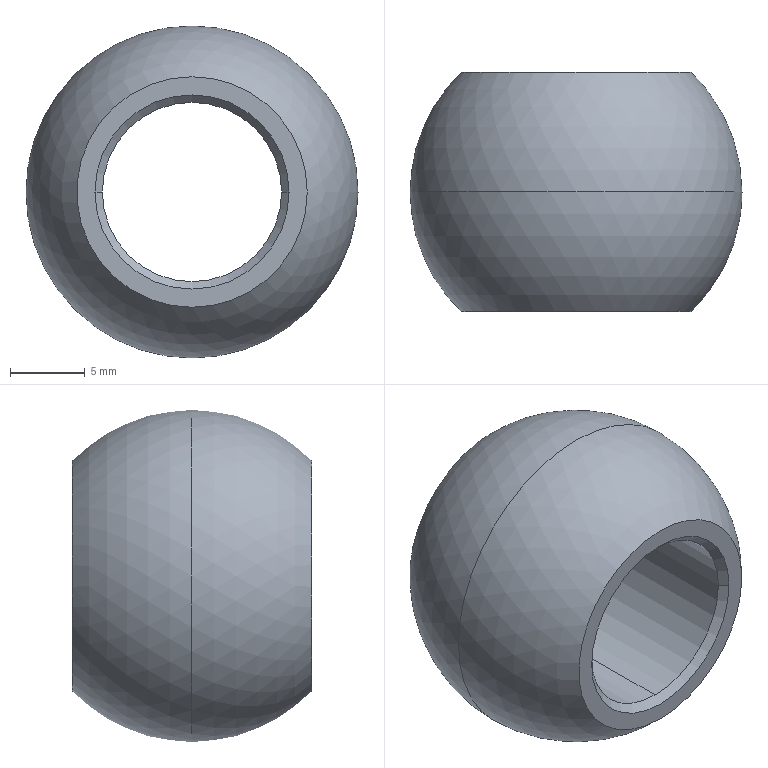Part | NX | 1 solid | 10 faces | box 22.225 x 16 x 22.225 mm | volume 3316 mm3 | cone 4 | cylinder 2 | sphere 2 | plane 2 | commonest cylinder face diameters 12 x2
STEP:
#1=CARTESIAN_POINT('',(6.,7.5,50.));
#2=VERTEX_POINT('',#1);
#3=CARTESIAN_POINT('',(0.,7.5,56.));
#4=VERTEX_POINT('',#3);
#5=CARTESIAN_POINT('',(0.,7.5,50.));
#6=DIRECTION('',(0.,-1.,0.));
#7=DIRECTION('',(0.,0.,-1.));
#8=AXIS2_PLACEMENT_3D('',#5,#6,#7);
#9=CIRCLE('',#8,6.);
#10=EDGE_CURVE('',#2,#4,#9,.T.);
#11=ORIENTED_EDGE('',*,*,#10,.F.);
#12=CARTESIAN_POINT('',(0.,7.5,44.));
#13=VERTEX_POINT('',#12);
#14=CARTESIAN_POINT('',(0.,7.5,50.));
#15=DIRECTION('',(0.,-1.,0.));
#16=DIRECTION('',(0.,0.,-1.));
#17=AXIS2_PLACEMENT_3D('',#14,#15,#16);
#18=CIRCLE('',#17,6.);
#19=EDGE_CURVE('',#13,#2,#18,.T.);
#20=ORIENTED_EDGE('',*,*,#19,.F.);
#21=CARTESIAN_POINT('',(0.,-7.5,44.));
#22=VERTEX_POINT('',#21);
#23=CARTESIAN_POINT('',(0.,0.,44.));
#24=DIRECTION('',(0.,-1.,0.));
#25=VECTOR('',#24,1000.);
#26=LINE('',#23,#25);
#27=EDGE_CURVE('',#13,#22,#26,.T.);
#28=ORIENTED_EDGE('',*,*,#27,.T.);
#29=CARTESIAN_POINT('',(6.,-7.5,50.));
#30=VERTEX_POINT('',#29);
#31=CARTESIAN_POINT('',(0.,-7.5,50.));
#32=DIRECTION('',(0.,-1.,0.));
#33=DIRECTION('',(0.,0.,-1.));
#34=AXIS2_PLACEMENT_3D('',#31,#32,#33);
#35=CIRCLE('',#34,6.);
#36=EDGE_CURVE('',#22,#30,#35,.T.);
#37=ORIENTED_EDGE('',*,*,#36,.T.);
#38=CARTESIAN_POINT('',(0.,-7.5,56.));
#39=VERTEX_POINT('',#38);
#40=CARTESIAN_POINT('',(0.,-7.5,50.));
#41=DIRECTION('',(0.,-1.,0.));
#42=DIRECTION('',(0.,0.,-1.));
#43=AXIS2_PLACEMENT_3D('',#40,#41,#42);
#44=CIRCLE('',#43,6.);
#45=EDGE_CURVE('',#30,#39,#44,.T.);
#46=ORIENTED_EDGE('',*,*,#45,.T.);
#47=CARTESIAN_POINT('',(0.,0.,56.));
#48=DIRECTION('',(0.,-1.,0.));
#49=VECTOR('',#48,1000.);
#50=LINE('',#47,#49);
#51=EDGE_CURVE('',#4,#39,#50,.T.);
#52=ORIENTED_EDGE('',*,*,#51,.F.);
#53=EDGE_LOOP('',(#11,#20,#28,#37,#46,#52));
#54=FACE_BOUND('',#53,.T.);
#55=CARTESIAN_POINT('',(0.,0.,50.));
#56=DIRECTION('',(0.,-1.,0.));
#57=DIRECTION('',(0.,0.,-1.));
#58=AXIS2_PLACEMENT_3D('',#55,#56,#57);
#59=CYLINDRICAL_SURFACE('',#58,6.);
#60=ADVANCED_FACE('',(#54),#59,.F.);
#61=CARTESIAN_POINT('',(11.113,0.,50.));
#62=VERTEX_POINT('',#61);
#63=CARTESIAN_POINT('',(-11.113,0.,50.));
#64=VERTEX_POINT('',#63);
#65=CARTESIAN_POINT('',(0.,0.,50.));
#66=DIRECTION('',(0.,1.,0.));
#67=DIRECTION('',(1.,0.,0.));
#68=AXIS2_PLACEMENT_3D('',#65,#66,#67);
#69=CIRCLE('',#68,11.113);
#70=EDGE_CURVE('',#62,#64,#69,.T.);
#71=ORIENTED_EDGE('',*,*,#70,.T.);
#72=CARTESIAN_POINT('',(0.,0.,50.));
#73=DIRECTION('',(0.,1.,0.));
#74=DIRECTION('',(1.,0.,0.));
#75=AXIS2_PLACEMENT_3D('',#72,#73,#74);
#76=CIRCLE('',#75,11.113);
#77=EDGE_CURVE('',#64,#62,#76,.T.);
#78=ORIENTED_EDGE('',*,*,#77,.T.);
#79=EDGE_LOOP('',(#71,#78));
#80=FACE_BOUND('',#79,.T.);
#81=CARTESIAN_POINT('',(0.,8.,57.713));
#82=VERTEX_POINT('',#81);
#83=CARTESIAN_POINT('',(0.,8.,42.287));
#84=VERTEX_POINT('',#83);
#85=CARTESIAN_POINT('',(0.,8.,50.));
#86=DIRECTION('',(0.,-1.,0.));
#87=DIRECTION('',(0.,0.,1.));
#88=AXIS2_PLACEMENT_3D('',#85,#86,#87);
#89=CIRCLE('',#88,7.713);
#90=EDGE_CURVE('',#82,#84,#89,.T.);
#91=ORIENTED_EDGE('',*,*,#90,.T.);
#92=CARTESIAN_POINT('',(0.,8.,50.));
#93=DIRECTION('',(0.,-1.,0.));
#94=DIRECTION('',(0.,0.,1.));
#95=AXIS2_PLACEMENT_3D('',#92,#93,#94);
#96=CIRCLE('',#95,7.713);
#97=EDGE_CURVE('',#84,#82,#96,.T.);
#98=ORIENTED_EDGE('',*,*,#97,.T.);
#99=EDGE_LOOP('',(#91,#98));
#100=FACE_BOUND('',#99,.T.);
#101=CARTESIAN_POINT('',(0.,0.,50.));
#102=DIRECTION('',(0.,1.,0.));
#103=DIRECTION('',(1.,0.,0.));
#104=AXIS2_PLACEMENT_3D('',#101,#102,#103);
#105=SPHERICAL_SURFACE('',#104,11.113);
#106=ADVANCED_FACE('',(#80,#100),#105,.T.);
#107=CARTESIAN_POINT('',(-6.5,-8.,50.));
#108=VERTEX_POINT('',#107);
#109=CARTESIAN_POINT('',(6.5,-8.,50.));
#110=VERTEX_POINT('',#109);
#111=CARTESIAN_POINT('',(0.,-8.,50.));
#112=DIRECTION('',(0.,1.,0.));
#113=DIRECTION('',(0.,0.,-1.));
#114=AXIS2_PLACEMENT_3D('',#111,#112,#113);
#115=CIRCLE('',#114,6.5);
#116=EDGE_CURVE('',#108,#110,#115,.T.);
#117=ORIENTED_EDGE('',*,*,#116,.F.);
#118=CARTESIAN_POINT('',(-6.,-7.5,50.));
#119=VERTEX_POINT('',#118);
#120=CARTESIAN_POINT('',(-6.25,-7.75,50.));
#121=DIRECTION('',(-0.7071,-0.7071,0.));
#122=VECTOR('',#121,1000.);
#123=LINE('',#120,#122);
#124=EDGE_CURVE('',#108,#119,#123,.F.);
#125=ORIENTED_EDGE('',*,*,#124,.T.);
#126=CARTESIAN_POINT('',(0.,-7.5,50.));
#127=DIRECTION('',(0.,-1.,0.));
#128=DIRECTION('',(0.,0.,-1.));
#129=AXIS2_PLACEMENT_3D('',#126,#127,#128);
#130=CIRCLE('',#129,6.);
#131=EDGE_CURVE('',#39,#119,#130,.T.);
#132=ORIENTED_EDGE('',*,*,#131,.F.);
#133=ORIENTED_EDGE('',*,*,#45,.F.);
#134=CARTESIAN_POINT('',(6.25,-7.75,50.));
#135=DIRECTION('',(0.7071,-0.7071,0.));
#136=VECTOR('',#135,1000.);
#137=LINE('',#134,#136);
#138=EDGE_CURVE('',#110,#30,#137,.F.);
#139=ORIENTED_EDGE('',*,*,#138,.F.);
#140=EDGE_LOOP('',(#117,#125,#132,#133,#139));
#141=FACE_BOUND('',#140,.T.);
#142=CARTESIAN_POINT('',(0.,-7.75,50.));
#143=DIRECTION('',(0.,-1.,0.));
#144=DIRECTION('',(-1.,0.,0.));
#145=AXIS2_PLACEMENT_3D('',#142,#143,#144);
#146=CONICAL_SURFACE('',#145,6.25,0.7854);
#147=ADVANCED_FACE('',(#141),#146,.F.);
#148=ORIENTED_EDGE('',*,*,#90,.F.);
#149=ORIENTED_EDGE('',*,*,#97,.F.);
#150=EDGE_LOOP('',(#148,#149));
#151=FACE_BOUND('',#150,.T.);
#152=CARTESIAN_POINT('',(6.5,8.,50.));
#153=VERTEX_POINT('',#152);
#154=CARTESIAN_POINT('',(-6.5,8.,50.));
#155=VERTEX_POINT('',#154);
#156=CARTESIAN_POINT('',(0.,8.,50.));
#157=DIRECTION('',(0.,-1.,0.));
#158=DIRECTION('',(0.,0.,-1.));
#159=AXIS2_PLACEMENT_3D('',#156,#157,#158);
#160=CIRCLE('',#159,6.5);
#161=EDGE_CURVE('',#153,#155,#160,.T.);
#162=ORIENTED_EDGE('',*,*,#161,.T.);
#163=CARTESIAN_POINT('',(0.,8.,50.));
#164=DIRECTION('',(0.,-1.,0.));
#165=DIRECTION('',(0.,0.,-1.));
#166=AXIS2_PLACEMENT_3D('',#163,#164,#165);
#167=CIRCLE('',#166,6.5);
#168=EDGE_CURVE('',#155,#153,#167,.T.);
#169=ORIENTED_EDGE('',*,*,#168,.T.);
#170=EDGE_LOOP('',(#162,#169));
#171=FACE_BOUND('',#170,.T.);
#172=CARTESIAN_POINT('',(0.,8.,50.));
#173=DIRECTION('',(0.,1.,0.));
#174=DIRECTION('',(1.,0.,0.));
#175=AXIS2_PLACEMENT_3D('',#172,#173,#174);
#176=PLANE('',#175);
#177=ADVANCED_FACE('',(#151,#171),#176,.T.);
#178=ORIENTED_EDGE('',*,*,#161,.F.);
#179=CARTESIAN_POINT('',(6.25,7.75,50.));
#180=DIRECTION('',(0.7071,0.7071,0.));
#181=VECTOR('',#180,1000.);
#182=LINE('',#179,#181);
#183=EDGE_CURVE('',#2,#153,#182,.T.);
#184=ORIENTED_EDGE('',*,*,#183,.F.);
#185=ORIENTED_EDGE('',*,*,#10,.T.);
#186=CARTESIAN_POINT('',(-6.,7.5,50.));
#187=VERTEX_POINT('',#186);
#188=CARTESIAN_POINT('',(0.,7.5,50.));
#189=DIRECTION('',(0.,-1.,0.));
#190=DIRECTION('',(0.,0.,-1.));
#191=AXIS2_PLACEMENT_3D('',#188,#189,#190);
#192=CIRCLE('',#191,6.);
#193=EDGE_CURVE('',#4,#187,#192,.T.);
#194=ORIENTED_EDGE('',*,*,#193,.T.);
#195=CARTESIAN_POINT('',(-6.25,7.75,50.));
#196=DIRECTION('',(-0.7071,0.7071,0.));
#197=VECTOR('',#196,1000.);
#198=LINE('',#195,#197);
#199=EDGE_CURVE('',#187,#155,#198,.T.);
#200=ORIENTED_EDGE('',*,*,#199,.T.);
#201=EDGE_LOOP('',(#178,#184,#185,#194,#200));
#202=FACE_BOUND('',#201,.T.);
#203=CARTESIAN_POINT('',(0.,7.75,50.));
#204=DIRECTION('',(0.,1.,0.));
#205=DIRECTION('',(1.,0.,0.));
#206=AXIS2_PLACEMENT_3D('',#203,#204,#205);
#207=CONICAL_SURFACE('',#206,6.25,0.7854);
#208=ADVANCED_FACE('',(#202),#207,.F.);
#209=CARTESIAN_POINT('',(0.,-8.,42.287));
#210=VERTEX_POINT('',#209);
#211=CARTESIAN_POINT('',(0.,-8.,57.713));
#212=VERTEX_POINT('',#211);
#213=CARTESIAN_POINT('',(0.,-8.,50.));
#214=DIRECTION('',(0.,1.,0.));
#215=DIRECTION('',(0.,0.,-1.));
#216=AXIS2_PLACEMENT_3D('',#213,#214,#215);
#217=CIRCLE('',#216,7.713);
#218=EDGE_CURVE('',#210,#212,#217,.T.);
#219=ORIENTED_EDGE('',*,*,#218,.F.);
#220=CARTESIAN_POINT('',(0.,-8.,50.));
#221=DIRECTION('',(0.,1.,0.));
#222=DIRECTION('',(0.,0.,-1.));
#223=AXIS2_PLACEMENT_3D('',#220,#221,#222);
#224=CIRCLE('',#223,7.713);
#225=EDGE_CURVE('',#212,#210,#224,.T.);
#226=ORIENTED_EDGE('',*,*,#225,.F.);
#227=EDGE_LOOP('',(#219,#226));
#228=FACE_BOUND('',#227,.T.);
#229=ORIENTED_EDGE('',*,*,#116,.T.);
#230=CARTESIAN_POINT('',(0.,-8.,50.));
#231=DIRECTION('',(0.,1.,0.));
#232=DIRECTION('',(0.,0.,-1.));
#233=AXIS2_PLACEMENT_3D('',#230,#231,#232);
#234=CIRCLE('',#233,6.5);
#235=EDGE_CURVE('',#110,#108,#234,.T.);
#236=ORIENTED_EDGE('',*,*,#235,.T.);
#237=EDGE_LOOP('',(#229,#236));
#238=FACE_BOUND('',#237,.T.);
#239=CARTESIAN_POINT('',(0.,-8.,50.));
#240=DIRECTION('',(0.,-1.,0.));
#241=DIRECTION('',(-1.,0.,0.));
#242=AXIS2_PLACEMENT_3D('',#239,#240,#241);
#243=PLANE('',#242);
#244=ADVANCED_FACE('',(#228,#238),#243,.T.);
#245=ORIENTED_EDGE('',*,*,#183,.T.);
#246=ORIENTED_EDGE('',*,*,#168,.F.);
#247=ORIENTED_EDGE('',*,*,#199,.F.);
#248=CARTESIAN_POINT('',(0.,7.5,50.));
#249=DIRECTION('',(0.,-1.,0.));
#250=DIRECTION('',(0.,0.,-1.));
#251=AXIS2_PLACEMENT_3D('',#248,#249,#250);
#252=CIRCLE('',#251,6.);
#253=EDGE_CURVE('',#187,#13,#252,.T.);
#254=ORIENTED_EDGE('',*,*,#253,.T.);
#255=ORIENTED_EDGE('',*,*,#19,.T.);
#256=EDGE_LOOP('',(#245,#246,#247,#254,#255));
#257=FACE_BOUND('',#256,.T.);
#258=CARTESIAN_POINT('',(0.,7.75,50.));
#259=DIRECTION('',(0.,1.,0.));
#260=DIRECTION('',(1.,0.,0.));
#261=AXIS2_PLACEMENT_3D('',#258,#259,#260);
#262=CONICAL_SURFACE('',#261,6.25,0.7854);
#263=ADVANCED_FACE('',(#257),#262,.F.);
#264=ORIENTED_EDGE('',*,*,#51,.T.);
#265=ORIENTED_EDGE('',*,*,#131,.T.);
#266=CARTESIAN_POINT('',(0.,-7.5,50.));
#267=DIRECTION('',(0.,-1.,0.));
#268=DIRECTION('',(0.,0.,-1.));
#269=AXIS2_PLACEMENT_3D('',#266,#267,#268);
#270=CIRCLE('',#269,6.);
#271=EDGE_CURVE('',#119,#22,#270,.T.);
#272=ORIENTED_EDGE('',*,*,#271,.T.);
#273=ORIENTED_EDGE('',*,*,#27,.F.);
#274=ORIENTED_EDGE('',*,*,#253,.F.);
#275=ORIENTED_EDGE('',*,*,#193,.F.);
#276=EDGE_LOOP('',(#264,#265,#272,#273,#274,#275));
#277=FACE_BOUND('',#276,.T.);
#278=CARTESIAN_POINT('',(0.,0.,50.));
#279=DIRECTION('',(0.,-1.,0.));
#280=DIRECTION('',(0.,0.,-1.));
#281=AXIS2_PLACEMENT_3D('',#278,#279,#280);
#282=CYLINDRICAL_SURFACE('',#281,6.);
#283=ADVANCED_FACE('',(#277),#282,.F.);
#284=ORIENTED_EDGE('',*,*,#36,.F.);
#285=ORIENTED_EDGE('',*,*,#271,.F.);
#286=ORIENTED_EDGE('',*,*,#124,.F.);
#287=ORIENTED_EDGE('',*,*,#235,.F.);
#288=ORIENTED_EDGE('',*,*,#138,.T.);
#289=EDGE_LOOP('',(#284,#285,#286,#287,#288));
#290=FACE_BOUND('',#289,.T.);
#291=CARTESIAN_POINT('',(0.,-7.75,50.));
#292=DIRECTION('',(0.,-1.,0.));
#293=DIRECTION('',(-1.,0.,0.));
#294=AXIS2_PLACEMENT_3D('',#291,#292,#293);
#295=CONICAL_SURFACE('',#294,6.25,0.7854);
#296=ADVANCED_FACE('',(#290),#295,.F.);
#297=ORIENTED_EDGE('',*,*,#70,.F.);
#298=ORIENTED_EDGE('',*,*,#77,.F.);
#299=EDGE_LOOP('',(#297,#298));
#300=FACE_BOUND('',#299,.T.);
#301=ORIENTED_EDGE('',*,*,#218,.T.);
#302=ORIENTED_EDGE('',*,*,#225,.T.);
#303=EDGE_LOOP('',(#301,#302));
#304=FACE_BOUND('',#303,.T.);
#305=CARTESIAN_POINT('',(0.,0.,50.));
#306=DIRECTION('',(0.,1.,0.));
#307=DIRECTION('',(1.,0.,0.));
#308=AXIS2_PLACEMENT_3D('',#305,#306,#307);
#309=SPHERICAL_SURFACE('',#308,11.113);
#310=ADVANCED_FACE('',(#300,#304),#309,.T.);
#311=CLOSED_SHELL('',(#60,#106,#147,#177,#208,#244,#263,#283,#296,#310));
#312=MANIFOLD_SOLID_BREP('',#311);
#313=(LENGTH_UNIT()NAMED_UNIT(*)SI_UNIT(.MILLI.,.METRE.));
#314=UNCERTAINTY_MEASURE_WITH_UNIT(LENGTH_MEASURE(0.00001),#313,'','');
#315=(NAMED_UNIT(*)PLANE_ANGLE_UNIT()SI_UNIT($,.RADIAN.));
#316=(NAMED_UNIT(*)SI_UNIT($,.STERADIAN.)SOLID_ANGLE_UNIT());
#317=(GEOMETRIC_REPRESENTATION_CONTEXT(3)GLOBAL_UNCERTAINTY_ASSIGNED_CONTEXT((#314))GLOBAL_UNIT_ASSIGNED_CONTEXT((#313,#315,#316))REPRESENTATION_CONTEXT('',''));
#318=ADVANCED_BREP_SHAPE_REPRESENTATION('',(#312),#317);